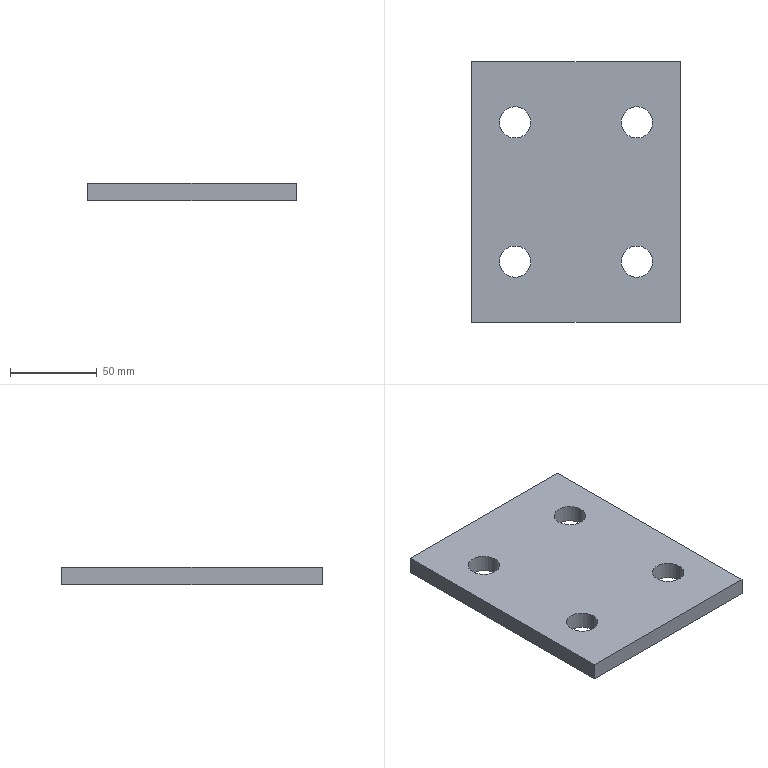Part | NX | features BREP 1 | 1 solid | 14 faces | box 120 x 150 x 10 mm | volume 169821 mm3 | cylinder 8 | plane 6 | commonest cylinder face diameters 18 x8
STEP:
#1=CARTESIAN_POINT('',(26.,40.,-5.));
#2=VERTEX_POINT('',#1);
#3=CARTESIAN_POINT('',(44.,40.,-5.));
#4=VERTEX_POINT('',#3);
#5=CARTESIAN_POINT('',(35.,40.,-5.));
#6=DIRECTION('',(0.,0.,1.));
#7=DIRECTION('',(-1.,0.,0.));
#8=AXIS2_PLACEMENT_3D('',#5,#6,#7);
#9=CIRCLE('',#8,9.);
#10=EDGE_CURVE('',#2,#4,#9,.T.);
#11=ORIENTED_EDGE('',*,*,#10,.F.);
#12=CARTESIAN_POINT('',(26.,40.,5.));
#13=VERTEX_POINT('',#12);
#14=CARTESIAN_POINT('',(26.,40.,-5.));
#15=DIRECTION('',(0.,0.,1.));
#16=VECTOR('',#15,1000.);
#17=LINE('',#14,#16);
#18=EDGE_CURVE('',#2,#13,#17,.T.);
#19=ORIENTED_EDGE('',*,*,#18,.T.);
#20=CARTESIAN_POINT('',(44.,40.,5.));
#21=VERTEX_POINT('',#20);
#22=CARTESIAN_POINT('',(35.,40.,5.));
#23=DIRECTION('',(0.,0.,1.));
#24=DIRECTION('',(-1.,0.,0.));
#25=AXIS2_PLACEMENT_3D('',#22,#23,#24);
#26=CIRCLE('',#25,9.);
#27=EDGE_CURVE('',#13,#21,#26,.T.);
#28=ORIENTED_EDGE('',*,*,#27,.T.);
#29=CARTESIAN_POINT('',(44.,40.,-5.));
#30=DIRECTION('',(0.,0.,1.));
#31=VECTOR('',#30,1000.);
#32=LINE('',#29,#31);
#33=EDGE_CURVE('',#4,#21,#32,.T.);
#34=ORIENTED_EDGE('',*,*,#33,.F.);
#35=EDGE_LOOP('',(#11,#19,#28,#34));
#36=FACE_BOUND('',#35,.T.);
#37=CARTESIAN_POINT('',(35.,40.,-5.));
#38=DIRECTION('',(0.,0.,1.));
#39=DIRECTION('',(-1.,0.,0.));
#40=AXIS2_PLACEMENT_3D('',#37,#38,#39);
#41=CYLINDRICAL_SURFACE('',#40,9.);
#42=ADVANCED_FACE('',(#36),#41,.F.);
#43=CARTESIAN_POINT('',(26.,-40.,-5.));
#44=VERTEX_POINT('',#43);
#45=CARTESIAN_POINT('',(44.,-40.,-5.));
#46=VERTEX_POINT('',#45);
#47=CARTESIAN_POINT('',(35.,-40.,-5.));
#48=DIRECTION('',(0.,0.,1.));
#49=DIRECTION('',(1.,0.,0.));
#50=AXIS2_PLACEMENT_3D('',#47,#48,#49);
#51=CIRCLE('',#50,9.);
#52=EDGE_CURVE('',#44,#46,#51,.T.);
#53=ORIENTED_EDGE('',*,*,#52,.F.);
#54=CARTESIAN_POINT('',(26.,-40.,5.));
#55=VERTEX_POINT('',#54);
#56=CARTESIAN_POINT('',(26.,-40.,-5.));
#57=DIRECTION('',(0.,0.,1.));
#58=VECTOR('',#57,1000.);
#59=LINE('',#56,#58);
#60=EDGE_CURVE('',#44,#55,#59,.T.);
#61=ORIENTED_EDGE('',*,*,#60,.T.);
#62=CARTESIAN_POINT('',(44.,-40.,5.));
#63=VERTEX_POINT('',#62);
#64=CARTESIAN_POINT('',(35.,-40.,5.));
#65=DIRECTION('',(0.,0.,1.));
#66=DIRECTION('',(1.,0.,0.));
#67=AXIS2_PLACEMENT_3D('',#64,#65,#66);
#68=CIRCLE('',#67,9.);
#69=EDGE_CURVE('',#55,#63,#68,.T.);
#70=ORIENTED_EDGE('',*,*,#69,.T.);
#71=CARTESIAN_POINT('',(44.,-40.,-5.));
#72=DIRECTION('',(0.,0.,1.));
#73=VECTOR('',#72,1000.);
#74=LINE('',#71,#73);
#75=EDGE_CURVE('',#46,#63,#74,.T.);
#76=ORIENTED_EDGE('',*,*,#75,.F.);
#77=EDGE_LOOP('',(#53,#61,#70,#76));
#78=FACE_BOUND('',#77,.T.);
#79=CARTESIAN_POINT('',(35.,-40.,-5.));
#80=DIRECTION('',(0.,0.,1.));
#81=DIRECTION('',(-1.,0.,0.));
#82=AXIS2_PLACEMENT_3D('',#79,#80,#81);
#83=CYLINDRICAL_SURFACE('',#82,9.);
#84=ADVANCED_FACE('',(#78),#83,.F.);
#85=CARTESIAN_POINT('',(-44.,-40.,-5.));
#86=VERTEX_POINT('',#85);
#87=CARTESIAN_POINT('',(-26.,-40.,-5.));
#88=VERTEX_POINT('',#87);
#89=CARTESIAN_POINT('',(-35.,-40.,-5.));
#90=DIRECTION('',(0.,0.,1.));
#91=DIRECTION('',(-1.,0.,0.));
#92=AXIS2_PLACEMENT_3D('',#89,#90,#91);
#93=CIRCLE('',#92,9.);
#94=EDGE_CURVE('',#86,#88,#93,.T.);
#95=ORIENTED_EDGE('',*,*,#94,.F.);
#96=CARTESIAN_POINT('',(-44.,-40.,5.));
#97=VERTEX_POINT('',#96);
#98=CARTESIAN_POINT('',(-44.,-40.,-5.));
#99=DIRECTION('',(0.,0.,1.));
#100=VECTOR('',#99,1000.);
#101=LINE('',#98,#100);
#102=EDGE_CURVE('',#86,#97,#101,.T.);
#103=ORIENTED_EDGE('',*,*,#102,.T.);
#104=CARTESIAN_POINT('',(-26.,-40.,5.));
#105=VERTEX_POINT('',#104);
#106=CARTESIAN_POINT('',(-35.,-40.,5.));
#107=DIRECTION('',(0.,0.,1.));
#108=DIRECTION('',(-1.,0.,0.));
#109=AXIS2_PLACEMENT_3D('',#106,#107,#108);
#110=CIRCLE('',#109,9.);
#111=EDGE_CURVE('',#97,#105,#110,.T.);
#112=ORIENTED_EDGE('',*,*,#111,.T.);
#113=CARTESIAN_POINT('',(-26.,-40.,-5.));
#114=DIRECTION('',(0.,0.,1.));
#115=VECTOR('',#114,1000.);
#116=LINE('',#113,#115);
#117=EDGE_CURVE('',#88,#105,#116,.T.);
#118=ORIENTED_EDGE('',*,*,#117,.F.);
#119=EDGE_LOOP('',(#95,#103,#112,#118));
#120=FACE_BOUND('',#119,.T.);
#121=CARTESIAN_POINT('',(-35.,-40.,-5.));
#122=DIRECTION('',(0.,0.,1.));
#123=DIRECTION('',(-1.,0.,0.));
#124=AXIS2_PLACEMENT_3D('',#121,#122,#123);
#125=CYLINDRICAL_SURFACE('',#124,9.);
#126=ADVANCED_FACE('',(#120),#125,.F.);
#127=CARTESIAN_POINT('',(-44.,40.,-5.));
#128=VERTEX_POINT('',#127);
#129=CARTESIAN_POINT('',(-26.,40.,-5.));
#130=VERTEX_POINT('',#129);
#131=CARTESIAN_POINT('',(-35.,40.,-5.));
#132=DIRECTION('',(0.,0.,1.));
#133=DIRECTION('',(1.,0.,0.));
#134=AXIS2_PLACEMENT_3D('',#131,#132,#133);
#135=CIRCLE('',#134,9.);
#136=EDGE_CURVE('',#128,#130,#135,.T.);
#137=ORIENTED_EDGE('',*,*,#136,.F.);
#138=CARTESIAN_POINT('',(-44.,40.,5.));
#139=VERTEX_POINT('',#138);
#140=CARTESIAN_POINT('',(-44.,40.,-5.));
#141=DIRECTION('',(0.,0.,1.));
#142=VECTOR('',#141,1000.);
#143=LINE('',#140,#142);
#144=EDGE_CURVE('',#128,#139,#143,.T.);
#145=ORIENTED_EDGE('',*,*,#144,.T.);
#146=CARTESIAN_POINT('',(-26.,40.,5.));
#147=VERTEX_POINT('',#146);
#148=CARTESIAN_POINT('',(-35.,40.,5.));
#149=DIRECTION('',(0.,0.,1.));
#150=DIRECTION('',(1.,0.,0.));
#151=AXIS2_PLACEMENT_3D('',#148,#149,#150);
#152=CIRCLE('',#151,9.);
#153=EDGE_CURVE('',#139,#147,#152,.T.);
#154=ORIENTED_EDGE('',*,*,#153,.T.);
#155=CARTESIAN_POINT('',(-26.,40.,-5.));
#156=DIRECTION('',(0.,0.,1.));
#157=VECTOR('',#156,1000.);
#158=LINE('',#155,#157);
#159=EDGE_CURVE('',#130,#147,#158,.T.);
#160=ORIENTED_EDGE('',*,*,#159,.F.);
#161=EDGE_LOOP('',(#137,#145,#154,#160));
#162=FACE_BOUND('',#161,.T.);
#163=CARTESIAN_POINT('',(-35.,40.,-5.));
#164=DIRECTION('',(0.,0.,1.));
#165=DIRECTION('',(-1.,0.,0.));
#166=AXIS2_PLACEMENT_3D('',#163,#164,#165);
#167=CYLINDRICAL_SURFACE('',#166,9.);
#168=ADVANCED_FACE('',(#162),#167,.F.);
#169=CARTESIAN_POINT('',(-60.,75.,-5.));
#170=VERTEX_POINT('',#169);
#171=CARTESIAN_POINT('',(-60.,-75.,-5.));
#172=VERTEX_POINT('',#171);
#173=CARTESIAN_POINT('',(-60.,75.,-5.));
#174=DIRECTION('',(0.,-1.,0.));
#175=VECTOR('',#174,1000.);
#176=LINE('',#173,#175);
#177=EDGE_CURVE('',#170,#172,#176,.T.);
#178=ORIENTED_EDGE('',*,*,#177,.T.);
#179=CARTESIAN_POINT('',(-60.,-75.,5.));
#180=VERTEX_POINT('',#179);
#181=CARTESIAN_POINT('',(-60.,-75.,5.));
#182=DIRECTION('',(0.,0.,-1.));
#183=VECTOR('',#182,1000.);
#184=LINE('',#181,#183);
#185=EDGE_CURVE('',#180,#172,#184,.T.);
#186=ORIENTED_EDGE('',*,*,#185,.F.);
#187=CARTESIAN_POINT('',(-60.,75.,5.));
#188=VERTEX_POINT('',#187);
#189=CARTESIAN_POINT('',(-60.,75.,5.));
#190=DIRECTION('',(0.,-1.,0.));
#191=VECTOR('',#190,1000.);
#192=LINE('',#189,#191);
#193=EDGE_CURVE('',#188,#180,#192,.T.);
#194=ORIENTED_EDGE('',*,*,#193,.F.);
#195=CARTESIAN_POINT('',(-60.,75.,5.));
#196=DIRECTION('',(0.,0.,-1.));
#197=VECTOR('',#196,1000.);
#198=LINE('',#195,#197);
#199=EDGE_CURVE('',#188,#170,#198,.T.);
#200=ORIENTED_EDGE('',*,*,#199,.T.);
#201=EDGE_LOOP('',(#178,#186,#194,#200));
#202=FACE_BOUND('',#201,.T.);
#203=CARTESIAN_POINT('',(-60.,75.,5.));
#204=DIRECTION('',(1.,0.,0.));
#205=DIRECTION('',(0.,0.,1.));
#206=AXIS2_PLACEMENT_3D('',#203,#204,#205);
#207=PLANE('',#206);
#208=ADVANCED_FACE('',(#202),#207,.F.);
#209=CARTESIAN_POINT('',(60.,-75.,-5.));
#210=VERTEX_POINT('',#209);
#211=CARTESIAN_POINT('',(-60.,-75.,-5.));
#212=DIRECTION('',(1.,0.,0.));
#213=VECTOR('',#212,1000.);
#214=LINE('',#211,#213);
#215=EDGE_CURVE('',#172,#210,#214,.T.);
#216=ORIENTED_EDGE('',*,*,#215,.T.);
#217=CARTESIAN_POINT('',(60.,-75.,5.));
#218=VERTEX_POINT('',#217);
#219=CARTESIAN_POINT('',(60.,-75.,5.));
#220=DIRECTION('',(0.,0.,-1.));
#221=VECTOR('',#220,1000.);
#222=LINE('',#219,#221);
#223=EDGE_CURVE('',#218,#210,#222,.T.);
#224=ORIENTED_EDGE('',*,*,#223,.F.);
#225=CARTESIAN_POINT('',(-60.,-75.,5.));
#226=DIRECTION('',(1.,0.,0.));
#227=VECTOR('',#226,1000.);
#228=LINE('',#225,#227);
#229=EDGE_CURVE('',#180,#218,#228,.T.);
#230=ORIENTED_EDGE('',*,*,#229,.F.);
#231=ORIENTED_EDGE('',*,*,#185,.T.);
#232=EDGE_LOOP('',(#216,#224,#230,#231));
#233=FACE_BOUND('',#232,.T.);
#234=CARTESIAN_POINT('',(-60.,-75.,5.));
#235=DIRECTION('',(0.,1.,0.));
#236=DIRECTION('',(0.,0.,-1.));
#237=AXIS2_PLACEMENT_3D('',#234,#235,#236);
#238=PLANE('',#237);
#239=ADVANCED_FACE('',(#233),#238,.F.);
#240=CARTESIAN_POINT('',(60.,75.,-5.));
#241=VERTEX_POINT('',#240);
#242=CARTESIAN_POINT('',(60.,75.,-5.));
#243=DIRECTION('',(0.,1.,0.));
#244=VECTOR('',#243,1000.);
#245=LINE('',#242,#244);
#246=EDGE_CURVE('',#210,#241,#245,.T.);
#247=ORIENTED_EDGE('',*,*,#246,.T.);
#248=CARTESIAN_POINT('',(60.,75.,5.));
#249=VERTEX_POINT('',#248);
#250=CARTESIAN_POINT('',(60.,75.,5.));
#251=DIRECTION('',(0.,0.,-1.));
#252=VECTOR('',#251,1000.);
#253=LINE('',#250,#252);
#254=EDGE_CURVE('',#249,#241,#253,.T.);
#255=ORIENTED_EDGE('',*,*,#254,.F.);
#256=CARTESIAN_POINT('',(60.,75.,5.));
#257=DIRECTION('',(0.,1.,0.));
#258=VECTOR('',#257,1000.);
#259=LINE('',#256,#258);
#260=EDGE_CURVE('',#218,#249,#259,.T.);
#261=ORIENTED_EDGE('',*,*,#260,.F.);
#262=ORIENTED_EDGE('',*,*,#223,.T.);
#263=EDGE_LOOP('',(#247,#255,#261,#262));
#264=FACE_BOUND('',#263,.T.);
#265=CARTESIAN_POINT('',(60.,75.,5.));
#266=DIRECTION('',(-1.,0.,0.));
#267=DIRECTION('',(0.,0.,-1.));
#268=AXIS2_PLACEMENT_3D('',#265,#266,#267);
#269=PLANE('',#268);
#270=ADVANCED_FACE('',(#264),#269,.F.);
#271=CARTESIAN_POINT('',(-60.,75.,-5.));
#272=DIRECTION('',(-1.,0.,0.));
#273=VECTOR('',#272,1000.);
#274=LINE('',#271,#273);
#275=EDGE_CURVE('',#241,#170,#274,.T.);
#276=ORIENTED_EDGE('',*,*,#275,.T.);
#277=ORIENTED_EDGE('',*,*,#199,.F.);
#278=CARTESIAN_POINT('',(-60.,75.,5.));
#279=DIRECTION('',(-1.,0.,0.));
#280=VECTOR('',#279,1000.);
#281=LINE('',#278,#280);
#282=EDGE_CURVE('',#249,#188,#281,.T.);
#283=ORIENTED_EDGE('',*,*,#282,.F.);
#284=ORIENTED_EDGE('',*,*,#254,.T.);
#285=EDGE_LOOP('',(#276,#277,#283,#284));
#286=FACE_BOUND('',#285,.T.);
#287=CARTESIAN_POINT('',(-60.,75.,5.));
#288=DIRECTION('',(0.,-1.,0.));
#289=DIRECTION('',(0.,0.,1.));
#290=AXIS2_PLACEMENT_3D('',#287,#288,#289);
#291=PLANE('',#290);
#292=ADVANCED_FACE('',(#286),#291,.F.);
#293=CARTESIAN_POINT('',(35.,40.,5.));
#294=DIRECTION('',(0.,0.,1.));
#295=DIRECTION('',(-1.,0.,0.));
#296=AXIS2_PLACEMENT_3D('',#293,#294,#295);
#297=CIRCLE('',#296,9.);
#298=EDGE_CURVE('',#21,#13,#297,.T.);
#299=ORIENTED_EDGE('',*,*,#298,.F.);
#300=ORIENTED_EDGE('',*,*,#27,.F.);
#301=EDGE_LOOP('',(#299,#300));
#302=FACE_BOUND('',#301,.T.);
#303=CARTESIAN_POINT('',(35.,-40.,5.));
#304=DIRECTION('',(0.,0.,1.));
#305=DIRECTION('',(1.,0.,0.));
#306=AXIS2_PLACEMENT_3D('',#303,#304,#305);
#307=CIRCLE('',#306,9.);
#308=EDGE_CURVE('',#63,#55,#307,.T.);
#309=ORIENTED_EDGE('',*,*,#308,.F.);
#310=ORIENTED_EDGE('',*,*,#69,.F.);
#311=EDGE_LOOP('',(#309,#310));
#312=FACE_BOUND('',#311,.T.);
#313=CARTESIAN_POINT('',(-35.,-40.,5.));
#314=DIRECTION('',(0.,0.,1.));
#315=DIRECTION('',(-1.,0.,0.));
#316=AXIS2_PLACEMENT_3D('',#313,#314,#315);
#317=CIRCLE('',#316,9.);
#318=EDGE_CURVE('',#105,#97,#317,.T.);
#319=ORIENTED_EDGE('',*,*,#318,.F.);
#320=ORIENTED_EDGE('',*,*,#111,.F.);
#321=EDGE_LOOP('',(#319,#320));
#322=FACE_BOUND('',#321,.T.);
#323=CARTESIAN_POINT('',(-35.,40.,5.));
#324=DIRECTION('',(0.,0.,1.));
#325=DIRECTION('',(1.,0.,0.));
#326=AXIS2_PLACEMENT_3D('',#323,#324,#325);
#327=CIRCLE('',#326,9.);
#328=EDGE_CURVE('',#147,#139,#327,.T.);
#329=ORIENTED_EDGE('',*,*,#328,.F.);
#330=ORIENTED_EDGE('',*,*,#153,.F.);
#331=EDGE_LOOP('',(#329,#330));
#332=FACE_BOUND('',#331,.T.);
#333=ORIENTED_EDGE('',*,*,#193,.T.);
#334=ORIENTED_EDGE('',*,*,#229,.T.);
#335=ORIENTED_EDGE('',*,*,#260,.T.);
#336=ORIENTED_EDGE('',*,*,#282,.T.);
#337=EDGE_LOOP('',(#333,#334,#335,#336));
#338=FACE_BOUND('',#337,.T.);
#339=CARTESIAN_POINT('',(-60.,-75.,5.));
#340=DIRECTION('',(0.,0.,1.));
#341=DIRECTION('',(-1.,0.,0.));
#342=AXIS2_PLACEMENT_3D('',#339,#340,#341);
#343=PLANE('',#342);
#344=ADVANCED_FACE('',(#302,#312,#322,#332,#338),#343,.T.);
#345=CARTESIAN_POINT('',(35.,40.,-5.));
#346=DIRECTION('',(0.,0.,1.));
#347=DIRECTION('',(-1.,0.,0.));
#348=AXIS2_PLACEMENT_3D('',#345,#346,#347);
#349=CIRCLE('',#348,9.);
#350=EDGE_CURVE('',#4,#2,#349,.T.);
#351=ORIENTED_EDGE('',*,*,#350,.T.);
#352=ORIENTED_EDGE('',*,*,#10,.T.);
#353=EDGE_LOOP('',(#351,#352));
#354=FACE_BOUND('',#353,.T.);
#355=CARTESIAN_POINT('',(35.,-40.,-5.));
#356=DIRECTION('',(0.,0.,1.));
#357=DIRECTION('',(1.,0.,0.));
#358=AXIS2_PLACEMENT_3D('',#355,#356,#357);
#359=CIRCLE('',#358,9.);
#360=EDGE_CURVE('',#46,#44,#359,.T.);
#361=ORIENTED_EDGE('',*,*,#360,.T.);
#362=ORIENTED_EDGE('',*,*,#52,.T.);
#363=EDGE_LOOP('',(#361,#362));
#364=FACE_BOUND('',#363,.T.);
#365=CARTESIAN_POINT('',(-35.,-40.,-5.));
#366=DIRECTION('',(0.,0.,1.));
#367=DIRECTION('',(-1.,0.,0.));
#368=AXIS2_PLACEMENT_3D('',#365,#366,#367);
#369=CIRCLE('',#368,9.);
#370=EDGE_CURVE('',#88,#86,#369,.T.);
#371=ORIENTED_EDGE('',*,*,#370,.T.);
#372=ORIENTED_EDGE('',*,*,#94,.T.);
#373=EDGE_LOOP('',(#371,#372));
#374=FACE_BOUND('',#373,.T.);
#375=CARTESIAN_POINT('',(-35.,40.,-5.));
#376=DIRECTION('',(0.,0.,1.));
#377=DIRECTION('',(1.,0.,0.));
#378=AXIS2_PLACEMENT_3D('',#375,#376,#377);
#379=CIRCLE('',#378,9.);
#380=EDGE_CURVE('',#130,#128,#379,.T.);
#381=ORIENTED_EDGE('',*,*,#380,.T.);
#382=ORIENTED_EDGE('',*,*,#136,.T.);
#383=EDGE_LOOP('',(#381,#382));
#384=FACE_BOUND('',#383,.T.);
#385=ORIENTED_EDGE('',*,*,#177,.F.);
#386=ORIENTED_EDGE('',*,*,#275,.F.);
#387=ORIENTED_EDGE('',*,*,#246,.F.);
#388=ORIENTED_EDGE('',*,*,#215,.F.);
#389=EDGE_LOOP('',(#385,#386,#387,#388));
#390=FACE_BOUND('',#389,.T.);
#391=CARTESIAN_POINT('',(-60.,-75.,-5.));
#392=DIRECTION('',(0.,0.,1.));
#393=DIRECTION('',(-1.,0.,0.));
#394=AXIS2_PLACEMENT_3D('',#391,#392,#393);
#395=PLANE('',#394);
#396=ADVANCED_FACE('',(#354,#364,#374,#384,#390),#395,.F.);
#397=ORIENTED_EDGE('',*,*,#144,.F.);
#398=ORIENTED_EDGE('',*,*,#380,.F.);
#399=ORIENTED_EDGE('',*,*,#159,.T.);
#400=ORIENTED_EDGE('',*,*,#328,.T.);
#401=EDGE_LOOP('',(#397,#398,#399,#400));
#402=FACE_BOUND('',#401,.T.);
#403=CARTESIAN_POINT('',(-35.,40.,-5.));
#404=DIRECTION('',(0.,0.,1.));
#405=DIRECTION('',(-1.,0.,0.));
#406=AXIS2_PLACEMENT_3D('',#403,#404,#405);
#407=CYLINDRICAL_SURFACE('',#406,9.);
#408=ADVANCED_FACE('',(#402),#407,.F.);
#409=ORIENTED_EDGE('',*,*,#102,.F.);
#410=ORIENTED_EDGE('',*,*,#370,.F.);
#411=ORIENTED_EDGE('',*,*,#117,.T.);
#412=ORIENTED_EDGE('',*,*,#318,.T.);
#413=EDGE_LOOP('',(#409,#410,#411,#412));
#414=FACE_BOUND('',#413,.T.);
#415=CARTESIAN_POINT('',(-35.,-40.,-5.));
#416=DIRECTION('',(0.,0.,1.));
#417=DIRECTION('',(-1.,0.,0.));
#418=AXIS2_PLACEMENT_3D('',#415,#416,#417);
#419=CYLINDRICAL_SURFACE('',#418,9.);
#420=ADVANCED_FACE('',(#414),#419,.F.);
#421=ORIENTED_EDGE('',*,*,#60,.F.);
#422=ORIENTED_EDGE('',*,*,#360,.F.);
#423=ORIENTED_EDGE('',*,*,#75,.T.);
#424=ORIENTED_EDGE('',*,*,#308,.T.);
#425=EDGE_LOOP('',(#421,#422,#423,#424));
#426=FACE_BOUND('',#425,.T.);
#427=CARTESIAN_POINT('',(35.,-40.,-5.));
#428=DIRECTION('',(0.,0.,1.));
#429=DIRECTION('',(-1.,0.,0.));
#430=AXIS2_PLACEMENT_3D('',#427,#428,#429);
#431=CYLINDRICAL_SURFACE('',#430,9.);
#432=ADVANCED_FACE('',(#426),#431,.F.);
#433=ORIENTED_EDGE('',*,*,#18,.F.);
#434=ORIENTED_EDGE('',*,*,#350,.F.);
#435=ORIENTED_EDGE('',*,*,#33,.T.);
#436=ORIENTED_EDGE('',*,*,#298,.T.);
#437=EDGE_LOOP('',(#433,#434,#435,#436));
#438=FACE_BOUND('',#437,.T.);
#439=CARTESIAN_POINT('',(35.,40.,-5.));
#440=DIRECTION('',(0.,0.,1.));
#441=DIRECTION('',(-1.,0.,0.));
#442=AXIS2_PLACEMENT_3D('',#439,#440,#441);
#443=CYLINDRICAL_SURFACE('',#442,9.);
#444=ADVANCED_FACE('',(#438),#443,.F.);
#445=CLOSED_SHELL('',(#42,#84,#126,#168,#208,#239,#270,#292,#344,#396,#408,#420,#432,#444));
#446=MANIFOLD_SOLID_BREP('',#445);
#447=(LENGTH_UNIT()NAMED_UNIT(*)SI_UNIT(.MILLI.,.METRE.));
#448=UNCERTAINTY_MEASURE_WITH_UNIT(LENGTH_MEASURE(0.00001),#447,'','');
#449=(NAMED_UNIT(*)PLANE_ANGLE_UNIT()SI_UNIT($,.RADIAN.));
#450=(NAMED_UNIT(*)SI_UNIT($,.STERADIAN.)SOLID_ANGLE_UNIT());
#451=(GEOMETRIC_REPRESENTATION_CONTEXT(3)GLOBAL_UNCERTAINTY_ASSIGNED_CONTEXT((#448))GLOBAL_UNIT_ASSIGNED_CONTEXT((#447,#449,#450))REPRESENTATION_CONTEXT('',''));
#452=ADVANCED_BREP_SHAPE_REPRESENTATION('',(#446),#451);